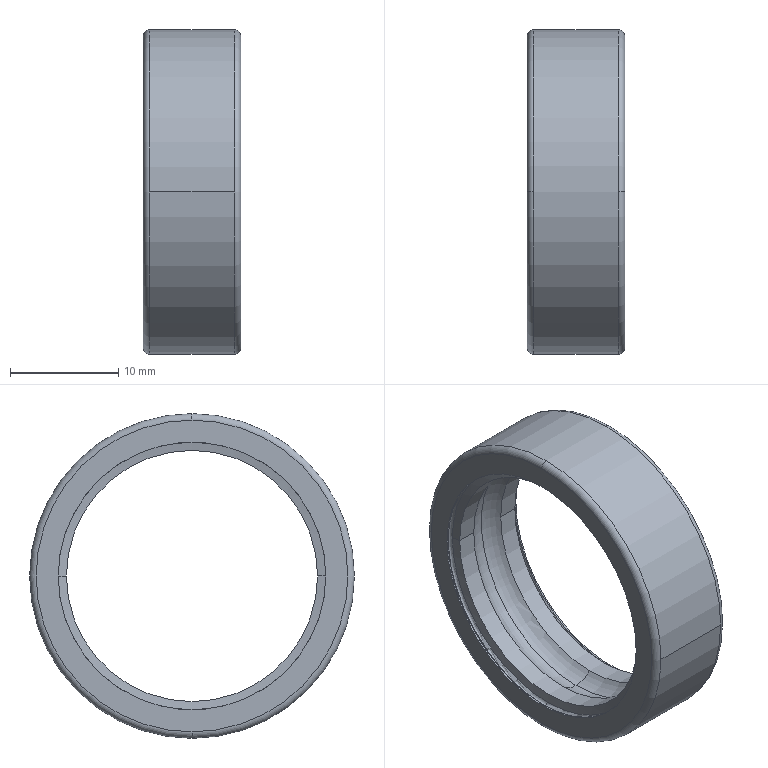Part | SolidWorks | features BaseBody 1 | 1 solid | 32 faces | box 9 x 30 x 30 mm | volume 2282 mm3 | torus 16 | cylinder 10 | cone 4 | plane 2 | commonest cylinder face diameters 23.2 x4 24.72 x4 30 x2
STEP:
#1=CARTESIAN_POINT('',(8.544,0.,-12.664));
#2=VERTEX_POINT('',#1);
#3=CARTESIAN_POINT('',(8.544,0.,12.664));
#4=VERTEX_POINT('',#3);
#5=CARTESIAN_POINT('',(8.544,0.,0.));
#6=DIRECTION('',(1.,0.,0.));
#7=DIRECTION('',(0.,0.,1.));
#8=AXIS2_PLACEMENT_3D('',#5,#6,#7);
#9=CIRCLE('',#8,12.664);
#10=EDGE_CURVE('',#2,#4,#9,.T.);
#11=ORIENTED_EDGE('',*,*,#10,.T.);
#12=CARTESIAN_POINT('',(8.245,0.,12.413));
#13=VERTEX_POINT('',#12);
#14=CARTESIAN_POINT('',(8.544,0.,12.36));
#15=DIRECTION('',(0.,-1.,0.));
#16=DIRECTION('',(0.,0.,1.));
#17=AXIS2_PLACEMENT_3D('',#14,#15,#16);
#18=CIRCLE('',#17,0.304);
#19=EDGE_CURVE('',#4,#13,#18,.T.);
#20=ORIENTED_EDGE('',*,*,#19,.T.);
#21=CARTESIAN_POINT('',(8.245,12.413,0.));
#22=VERTEX_POINT('',#21);
#23=CARTESIAN_POINT('',(8.245,0.,0.));
#24=DIRECTION('',(1.,0.,0.));
#25=DIRECTION('',(0.,1.,0.));
#26=AXIS2_PLACEMENT_3D('',#23,#24,#25);
#27=CIRCLE('',#26,12.413);
#28=EDGE_CURVE('',#22,#13,#27,.T.);
#29=ORIENTED_EDGE('',*,*,#28,.F.);
#30=CARTESIAN_POINT('',(8.245,0.,-12.413));
#31=VERTEX_POINT('',#30);
#32=CARTESIAN_POINT('',(8.245,0.,0.));
#33=DIRECTION('',(1.,0.,0.));
#34=DIRECTION('',(0.,1.,0.));
#35=AXIS2_PLACEMENT_3D('',#32,#33,#34);
#36=CIRCLE('',#35,12.413);
#37=EDGE_CURVE('',#31,#22,#36,.T.);
#38=ORIENTED_EDGE('',*,*,#37,.F.);
#39=CARTESIAN_POINT('',(8.544,0.,-12.36));
#40=DIRECTION('',(0.,-1.,0.));
#41=DIRECTION('',(0.,0.,-1.));
#42=AXIS2_PLACEMENT_3D('',#39,#40,#41);
#43=CIRCLE('',#42,0.304);
#44=EDGE_CURVE('',#31,#2,#43,.T.);
#45=ORIENTED_EDGE('',*,*,#44,.T.);
#46=EDGE_LOOP('',(#11,#20,#29,#38,#45));
#47=FACE_OUTER_BOUND('',#46,.T.);
#48=CARTESIAN_POINT('',(8.544,0.,0.));
#49=DIRECTION('',(1.,0.,0.));
#50=DIRECTION('',(0.,0.,-1.));
#51=AXIS2_PLACEMENT_3D('',#48,#49,#50);
#52=TOROIDAL_SURFACE('',#51,12.36,0.304);
#53=ADVANCED_FACE('',(#47),#52,.F.);
#54=CARTESIAN_POINT('',(8.848,12.36,0.));
#55=VERTEX_POINT('',#54);
#56=CARTESIAN_POINT('',(9.,12.36,0.));
#57=VERTEX_POINT('',#56);
#58=CARTESIAN_POINT('',(8.924,12.36,0.));
#59=DIRECTION('',(1.,0.,0.));
#60=VECTOR('',#59,1000.);
#61=LINE('',#58,#60);
#62=EDGE_CURVE('',#55,#57,#61,.T.);
#63=ORIENTED_EDGE('',*,*,#62,.T.);
#64=CARTESIAN_POINT('',(9.,-12.36,0.));
#65=VERTEX_POINT('',#64);
#66=CARTESIAN_POINT('',(9.,0.,0.));
#67=DIRECTION('',(1.,0.,0.));
#68=DIRECTION('',(0.,1.,0.));
#69=AXIS2_PLACEMENT_3D('',#66,#67,#68);
#70=CIRCLE('',#69,12.36);
#71=EDGE_CURVE('',#57,#65,#70,.T.);
#72=ORIENTED_EDGE('',*,*,#71,.T.);
#73=CARTESIAN_POINT('',(8.848,-12.36,0.));
#74=VERTEX_POINT('',#73);
#75=CARTESIAN_POINT('',(8.924,-12.36,0.));
#76=DIRECTION('',(-1.,0.,0.));
#77=VECTOR('',#76,1000.);
#78=LINE('',#75,#77);
#79=EDGE_CURVE('',#65,#74,#78,.T.);
#80=ORIENTED_EDGE('',*,*,#79,.T.);
#81=CARTESIAN_POINT('',(8.848,0.,12.36));
#82=VERTEX_POINT('',#81);
#83=CARTESIAN_POINT('',(8.848,0.,0.));
#84=DIRECTION('',(1.,0.,0.));
#85=DIRECTION('',(0.,1.,0.));
#86=AXIS2_PLACEMENT_3D('',#83,#84,#85);
#87=CIRCLE('',#86,12.36);
#88=EDGE_CURVE('',#82,#74,#87,.T.);
#89=ORIENTED_EDGE('',*,*,#88,.F.);
#90=CARTESIAN_POINT('',(8.848,0.,0.));
#91=DIRECTION('',(1.,0.,0.));
#92=DIRECTION('',(0.,1.,0.));
#93=AXIS2_PLACEMENT_3D('',#90,#91,#92);
#94=CIRCLE('',#93,12.36);
#95=EDGE_CURVE('',#55,#82,#94,.T.);
#96=ORIENTED_EDGE('',*,*,#95,.F.);
#97=EDGE_LOOP('',(#63,#72,#80,#89,#96));
#98=FACE_OUTER_BOUND('',#97,.T.);
#99=CARTESIAN_POINT('',(8.924,0.,0.));
#100=DIRECTION('',(1.,0.,0.));
#101=DIRECTION('',(0.,1.,0.));
#102=AXIS2_PLACEMENT_3D('',#99,#100,#101);
#103=CYLINDRICAL_SURFACE('',#102,12.36);
#104=ADVANCED_FACE('',(#98),#103,.F.);
#105=ORIENTED_EDGE('',*,*,#71,.F.);
#106=CARTESIAN_POINT('',(9.,0.,0.));
#107=DIRECTION('',(1.,0.,0.));
#108=DIRECTION('',(0.,1.,0.));
#109=AXIS2_PLACEMENT_3D('',#106,#107,#108);
#110=CIRCLE('',#109,12.36);
#111=EDGE_CURVE('',#65,#57,#110,.T.);
#112=ORIENTED_EDGE('',*,*,#111,.F.);
#113=EDGE_LOOP('',(#105,#112));
#114=FACE_BOUND('',#113,.T.);
#115=CARTESIAN_POINT('',(9.,0.,14.4));
#116=VERTEX_POINT('',#115);
#117=CARTESIAN_POINT('',(9.,0.,-14.4));
#118=VERTEX_POINT('',#117);
#119=CARTESIAN_POINT('',(9.,0.,0.));
#120=DIRECTION('',(1.,0.,0.));
#121=DIRECTION('',(0.,1.,0.));
#122=AXIS2_PLACEMENT_3D('',#119,#120,#121);
#123=CIRCLE('',#122,14.4);
#124=EDGE_CURVE('',#116,#118,#123,.T.);
#125=ORIENTED_EDGE('',*,*,#124,.T.);
#126=CARTESIAN_POINT('',(9.,0.,0.));
#127=DIRECTION('',(1.,0.,0.));
#128=DIRECTION('',(0.,1.,0.));
#129=AXIS2_PLACEMENT_3D('',#126,#127,#128);
#130=CIRCLE('',#129,14.4);
#131=EDGE_CURVE('',#118,#116,#130,.T.);
#132=ORIENTED_EDGE('',*,*,#131,.T.);
#133=EDGE_LOOP('',(#125,#132));
#134=FACE_OUTER_BOUND('',#133,.T.);
#135=CARTESIAN_POINT('',(9.,13.38,0.));
#136=DIRECTION('',(1.,0.,0.));
#137=DIRECTION('',(0.,1.,0.));
#138=AXIS2_PLACEMENT_3D('',#135,#136,#137);
#139=PLANE('',#138);
#140=ADVANCED_FACE('',(#114,#134),#139,.T.);
#141=CARTESIAN_POINT('',(8.4,0.,-15.));
#142=VERTEX_POINT('',#141);
#143=CARTESIAN_POINT('',(8.4,0.,-14.4));
#144=DIRECTION('',(0.,-1.,0.));
#145=DIRECTION('',(0.,0.,-1.));
#146=AXIS2_PLACEMENT_3D('',#143,#144,#145);
#147=CIRCLE('',#146,0.6);
#148=EDGE_CURVE('',#142,#118,#147,.T.);
#149=ORIENTED_EDGE('',*,*,#148,.T.);
#150=ORIENTED_EDGE('',*,*,#124,.F.);
#151=CARTESIAN_POINT('',(8.4,0.,15.));
#152=VERTEX_POINT('',#151);
#153=CARTESIAN_POINT('',(8.4,0.,14.4));
#154=DIRECTION('',(0.,-1.,0.));
#155=DIRECTION('',(0.,0.,1.));
#156=AXIS2_PLACEMENT_3D('',#153,#154,#155);
#157=CIRCLE('',#156,0.6);
#158=EDGE_CURVE('',#116,#152,#157,.T.);
#159=ORIENTED_EDGE('',*,*,#158,.T.);
#160=CARTESIAN_POINT('',(8.4,-15.,0.));
#161=VERTEX_POINT('',#160);
#162=CARTESIAN_POINT('',(8.4,0.,0.));
#163=DIRECTION('',(1.,0.,0.));
#164=DIRECTION('',(0.,1.,0.));
#165=AXIS2_PLACEMENT_3D('',#162,#163,#164);
#166=CIRCLE('',#165,15.);
#167=EDGE_CURVE('',#152,#161,#166,.T.);
#168=ORIENTED_EDGE('',*,*,#167,.T.);
#169=CARTESIAN_POINT('',(8.4,0.,0.));
#170=DIRECTION('',(1.,0.,0.));
#171=DIRECTION('',(0.,1.,0.));
#172=AXIS2_PLACEMENT_3D('',#169,#170,#171);
#173=CIRCLE('',#172,15.);
#174=EDGE_CURVE('',#161,#142,#173,.T.);
#175=ORIENTED_EDGE('',*,*,#174,.T.);
#176=EDGE_LOOP('',(#149,#150,#159,#168,#175));
#177=FACE_OUTER_BOUND('',#176,.T.);
#178=CARTESIAN_POINT('',(8.4,0.,0.));
#179=DIRECTION('',(1.,0.,0.));
#180=DIRECTION('',(0.,0.,-1.));
#181=AXIS2_PLACEMENT_3D('',#178,#179,#180);
#182=TOROIDAL_SURFACE('',#181,14.4,0.6);
#183=ADVANCED_FACE('',(#177),#182,.T.);
#184=CARTESIAN_POINT('',(0.6,15.,0.));
#185=VERTEX_POINT('',#184);
#186=CARTESIAN_POINT('',(8.4,15.,0.));
#187=VERTEX_POINT('',#186);
#188=CARTESIAN_POINT('',(4.5,15.,0.));
#189=DIRECTION('',(1.,0.,0.));
#190=VECTOR('',#189,1000.);
#191=LINE('',#188,#190);
#192=EDGE_CURVE('',#185,#187,#191,.T.);
#193=ORIENTED_EDGE('',*,*,#192,.T.);
#194=CARTESIAN_POINT('',(8.4,0.,0.));
#195=DIRECTION('',(1.,0.,0.));
#196=DIRECTION('',(0.,1.,0.));
#197=AXIS2_PLACEMENT_3D('',#194,#195,#196);
#198=CIRCLE('',#197,15.);
#199=EDGE_CURVE('',#142,#187,#198,.T.);
#200=ORIENTED_EDGE('',*,*,#199,.F.);
#201=ORIENTED_EDGE('',*,*,#174,.F.);
#202=CARTESIAN_POINT('',(0.6,-15.,0.));
#203=VERTEX_POINT('',#202);
#204=CARTESIAN_POINT('',(4.5,-15.,0.));
#205=DIRECTION('',(-1.,0.,0.));
#206=VECTOR('',#205,1000.);
#207=LINE('',#204,#206);
#208=EDGE_CURVE('',#161,#203,#207,.T.);
#209=ORIENTED_EDGE('',*,*,#208,.T.);
#210=CARTESIAN_POINT('',(0.6,0.,-15.));
#211=VERTEX_POINT('',#210);
#212=CARTESIAN_POINT('',(0.6,0.,0.));
#213=DIRECTION('',(1.,0.,0.));
#214=DIRECTION('',(0.,1.,0.));
#215=AXIS2_PLACEMENT_3D('',#212,#213,#214);
#216=CIRCLE('',#215,15.);
#217=EDGE_CURVE('',#203,#211,#216,.T.);
#218=ORIENTED_EDGE('',*,*,#217,.T.);
#219=CARTESIAN_POINT('',(0.6,0.,0.));
#220=DIRECTION('',(1.,0.,0.));
#221=DIRECTION('',(0.,1.,0.));
#222=AXIS2_PLACEMENT_3D('',#219,#220,#221);
#223=CIRCLE('',#222,15.);
#224=EDGE_CURVE('',#211,#185,#223,.T.);
#225=ORIENTED_EDGE('',*,*,#224,.T.);
#226=EDGE_LOOP('',(#193,#200,#201,#209,#218,#225));
#227=FACE_OUTER_BOUND('',#226,.T.);
#228=CARTESIAN_POINT('',(4.5,0.,0.));
#229=DIRECTION('',(1.,0.,0.));
#230=DIRECTION('',(0.,1.,0.));
#231=AXIS2_PLACEMENT_3D('',#228,#229,#230);
#232=CYLINDRICAL_SURFACE('',#231,15.);
#233=ADVANCED_FACE('',(#227),#232,.T.);
#234=CARTESIAN_POINT('',(0.,0.,-14.4));
#235=VERTEX_POINT('',#234);
#236=CARTESIAN_POINT('',(0.6,0.,-14.4));
#237=DIRECTION('',(0.,-1.,0.));
#238=DIRECTION('',(0.,0.,-1.));
#239=AXIS2_PLACEMENT_3D('',#236,#237,#238);
#240=CIRCLE('',#239,0.6);
#241=EDGE_CURVE('',#235,#211,#240,.T.);
#242=ORIENTED_EDGE('',*,*,#241,.T.);
#243=ORIENTED_EDGE('',*,*,#217,.F.);
#244=CARTESIAN_POINT('',(0.6,0.,15.));
#245=VERTEX_POINT('',#244);
#246=CARTESIAN_POINT('',(0.6,0.,0.));
#247=DIRECTION('',(1.,0.,0.));
#248=DIRECTION('',(0.,1.,0.));
#249=AXIS2_PLACEMENT_3D('',#246,#247,#248);
#250=CIRCLE('',#249,15.);
#251=EDGE_CURVE('',#245,#203,#250,.T.);
#252=ORIENTED_EDGE('',*,*,#251,.F.);
#253=CARTESIAN_POINT('',(0.,0.,14.4));
#254=VERTEX_POINT('',#253);
#255=CARTESIAN_POINT('',(0.6,0.,14.4));
#256=DIRECTION('',(0.,-1.,0.));
#257=DIRECTION('',(0.,0.,1.));
#258=AXIS2_PLACEMENT_3D('',#255,#256,#257);
#259=CIRCLE('',#258,0.6);
#260=EDGE_CURVE('',#245,#254,#259,.T.);
#261=ORIENTED_EDGE('',*,*,#260,.T.);
#262=CARTESIAN_POINT('',(0.,0.,0.));
#263=DIRECTION('',(1.,0.,0.));
#264=DIRECTION('',(0.,1.,0.));
#265=AXIS2_PLACEMENT_3D('',#262,#263,#264);
#266=CIRCLE('',#265,14.4);
#267=EDGE_CURVE('',#254,#235,#266,.T.);
#268=ORIENTED_EDGE('',*,*,#267,.T.);
#269=EDGE_LOOP('',(#242,#243,#252,#261,#268));
#270=FACE_OUTER_BOUND('',#269,.T.);
#271=CARTESIAN_POINT('',(0.6,0.,0.));
#272=DIRECTION('',(1.,0.,0.));
#273=DIRECTION('',(0.,0.,-1.));
#274=AXIS2_PLACEMENT_3D('',#271,#272,#273);
#275=TOROIDAL_SURFACE('',#274,14.4,0.6);
#276=ADVANCED_FACE('',(#270),#275,.T.);
#277=CARTESIAN_POINT('',(0.,12.36,0.));
#278=VERTEX_POINT('',#277);
#279=CARTESIAN_POINT('',(0.,-12.36,0.));
#280=VERTEX_POINT('',#279);
#281=CARTESIAN_POINT('',(0.,0.,0.));
#282=DIRECTION('',(1.,0.,0.));
#283=DIRECTION('',(0.,1.,0.));
#284=AXIS2_PLACEMENT_3D('',#281,#282,#283);
#285=CIRCLE('',#284,12.36);
#286=EDGE_CURVE('',#278,#280,#285,.T.);
#287=ORIENTED_EDGE('',*,*,#286,.T.);
#288=CARTESIAN_POINT('',(0.,0.,0.));
#289=DIRECTION('',(1.,0.,0.));
#290=DIRECTION('',(0.,1.,0.));
#291=AXIS2_PLACEMENT_3D('',#288,#289,#290);
#292=CIRCLE('',#291,12.36);
#293=EDGE_CURVE('',#280,#278,#292,.T.);
#294=ORIENTED_EDGE('',*,*,#293,.T.);
#295=EDGE_LOOP('',(#287,#294));
#296=FACE_BOUND('',#295,.T.);
#297=CARTESIAN_POINT('',(0.,0.,0.));
#298=DIRECTION('',(1.,0.,0.));
#299=DIRECTION('',(0.,1.,0.));
#300=AXIS2_PLACEMENT_3D('',#297,#298,#299);
#301=CIRCLE('',#300,14.4);
#302=EDGE_CURVE('',#235,#254,#301,.T.);
#303=ORIENTED_EDGE('',*,*,#302,.F.);
#304=ORIENTED_EDGE('',*,*,#267,.F.);
#305=EDGE_LOOP('',(#303,#304));
#306=FACE_OUTER_BOUND('',#305,.T.);
#307=CARTESIAN_POINT('',(0.,13.38,0.));
#308=DIRECTION('',(-1.,0.,0.));
#309=DIRECTION('',(0.,0.,1.));
#310=AXIS2_PLACEMENT_3D('',#307,#308,#309);
#311=PLANE('',#310);
#312=ADVANCED_FACE('',(#296,#306),#311,.T.);
#313=CARTESIAN_POINT('',(0.152,12.36,0.));
#314=VERTEX_POINT('',#313);
#315=CARTESIAN_POINT('',(0.076,12.36,0.));
#316=DIRECTION('',(1.,0.,0.));
#317=VECTOR('',#316,1000.);
#318=LINE('',#315,#317);
#319=EDGE_CURVE('',#278,#314,#318,.T.);
#320=ORIENTED_EDGE('',*,*,#319,.T.);
#321=CARTESIAN_POINT('',(0.152,0.,12.36));
#322=VERTEX_POINT('',#321);
#323=CARTESIAN_POINT('',(0.152,0.,0.));
#324=DIRECTION('',(1.,0.,0.));
#325=DIRECTION('',(0.,1.,0.));
#326=AXIS2_PLACEMENT_3D('',#323,#324,#325);
#327=CIRCLE('',#326,12.36);
#328=EDGE_CURVE('',#314,#322,#327,.T.);
#329=ORIENTED_EDGE('',*,*,#328,.T.);
#330=CARTESIAN_POINT('',(0.152,-12.36,0.));
#331=VERTEX_POINT('',#330);
#332=CARTESIAN_POINT('',(0.152,0.,0.));
#333=DIRECTION('',(1.,0.,0.));
#334=DIRECTION('',(0.,1.,0.));
#335=AXIS2_PLACEMENT_3D('',#332,#333,#334);
#336=CIRCLE('',#335,12.36);
#337=EDGE_CURVE('',#322,#331,#336,.T.);
#338=ORIENTED_EDGE('',*,*,#337,.T.);
#339=CARTESIAN_POINT('',(0.076,-12.36,0.));
#340=DIRECTION('',(-1.,0.,0.));
#341=VECTOR('',#340,1000.);
#342=LINE('',#339,#341);
#343=EDGE_CURVE('',#331,#280,#342,.T.);
#344=ORIENTED_EDGE('',*,*,#343,.T.);
#345=ORIENTED_EDGE('',*,*,#286,.F.);
#346=EDGE_LOOP('',(#320,#329,#338,#344,#345));
#347=FACE_OUTER_BOUND('',#346,.T.);
#348=CARTESIAN_POINT('',(0.076,0.,0.));
#349=DIRECTION('',(1.,0.,0.));
#350=DIRECTION('',(0.,1.,0.));
#351=AXIS2_PLACEMENT_3D('',#348,#349,#350);
#352=CYLINDRICAL_SURFACE('',#351,12.36);
#353=ADVANCED_FACE('',(#347),#352,.F.);
#354=CARTESIAN_POINT('',(0.456,0.,-12.664));
#355=VERTEX_POINT('',#354);
#356=CARTESIAN_POINT('',(0.456,0.,12.664));
#357=VERTEX_POINT('',#356);
#358=CARTESIAN_POINT('',(0.456,0.,0.));
#359=DIRECTION('',(1.,0.,0.));
#360=DIRECTION('',(0.,0.,1.));
#361=AXIS2_PLACEMENT_3D('',#358,#359,#360);
#362=CIRCLE('',#361,12.664);
#363=EDGE_CURVE('',#355,#357,#362,.T.);
#364=ORIENTED_EDGE('',*,*,#363,.T.);
#365=CARTESIAN_POINT('',(0.456,0.,12.36));
#366=DIRECTION('',(0.,-1.,0.));
#367=DIRECTION('',(0.,0.,1.));
#368=AXIS2_PLACEMENT_3D('',#365,#366,#367);
#369=CIRCLE('',#368,0.304);
#370=EDGE_CURVE('',#357,#322,#369,.T.);
#371=ORIENTED_EDGE('',*,*,#370,.T.);
#372=ORIENTED_EDGE('',*,*,#328,.F.);
#373=CARTESIAN_POINT('',(0.152,0.,-12.36));
#374=VERTEX_POINT('',#373);
#375=CARTESIAN_POINT('',(0.152,0.,0.));
#376=DIRECTION('',(1.,0.,0.));
#377=DIRECTION('',(0.,1.,0.));
#378=AXIS2_PLACEMENT_3D('',#375,#376,#377);
#379=CIRCLE('',#378,12.36);
#380=EDGE_CURVE('',#374,#314,#379,.T.);
#381=ORIENTED_EDGE('',*,*,#380,.F.);
#382=CARTESIAN_POINT('',(0.456,0.,-12.36));
#383=DIRECTION('',(0.,-1.,0.));
#384=DIRECTION('',(0.,0.,-1.));
#385=AXIS2_PLACEMENT_3D('',#382,#383,#384);
#386=CIRCLE('',#385,0.304);
#387=EDGE_CURVE('',#374,#355,#386,.T.);
#388=ORIENTED_EDGE('',*,*,#387,.T.);
#389=EDGE_LOOP('',(#364,#371,#372,#381,#388));
#390=FACE_OUTER_BOUND('',#389,.T.);
#391=CARTESIAN_POINT('',(0.456,0.,0.));
#392=DIRECTION('',(1.,0.,0.));
#393=DIRECTION('',(0.,0.,-1.));
#394=AXIS2_PLACEMENT_3D('',#391,#392,#393);
#395=TOROIDAL_SURFACE('',#394,12.36,0.304);
#396=ADVANCED_FACE('',(#390),#395,.F.);
#397=CARTESIAN_POINT('',(0.7554,12.413,0.));
#398=VERTEX_POINT('',#397);
#399=CARTESIAN_POINT('',(0.8987,11.6,0.));
#400=VERTEX_POINT('',#399);
#401=CARTESIAN_POINT('',(0.827,12.006,0.));
#402=DIRECTION('',(0.1736,-0.9848,0.));
#403=VECTOR('',#402,1000.);
#404=LINE('',#401,#403);
#405=EDGE_CURVE('',#398,#400,#404,.T.);
#406=ORIENTED_EDGE('',*,*,#405,.T.);
#407=CARTESIAN_POINT('',(0.8987,-11.6,0.));
#408=VERTEX_POINT('',#407);
#409=CARTESIAN_POINT('',(0.8987,0.,0.));
#410=DIRECTION('',(1.,0.,0.));
#411=DIRECTION('',(0.,1.,0.));
#412=AXIS2_PLACEMENT_3D('',#409,#410,#411);
#413=CIRCLE('',#412,11.6);
#414=EDGE_CURVE('',#400,#408,#413,.T.);
#415=ORIENTED_EDGE('',*,*,#414,.T.);
#416=CARTESIAN_POINT('',(0.7554,-12.413,0.));
#417=VERTEX_POINT('',#416);
#418=CARTESIAN_POINT('',(0.827,-12.006,0.));
#419=DIRECTION('',(-0.1736,-0.9848,0.));
#420=VECTOR('',#419,1000.);
#421=LINE('',#418,#420);
#422=EDGE_CURVE('',#408,#417,#421,.T.);
#423=ORIENTED_EDGE('',*,*,#422,.T.);
#424=CARTESIAN_POINT('',(0.7554,0.,12.413));
#425=VERTEX_POINT('',#424);
#426=CARTESIAN_POINT('',(0.7554,0.,0.));
#427=DIRECTION('',(1.,0.,0.));
#428=DIRECTION('',(0.,1.,0.));
#429=AXIS2_PLACEMENT_3D('',#426,#427,#428);
#430=CIRCLE('',#429,12.413);
#431=EDGE_CURVE('',#425,#417,#430,.T.);
#432=ORIENTED_EDGE('',*,*,#431,.F.);
#433=CARTESIAN_POINT('',(0.7554,0.,0.));
#434=DIRECTION('',(1.,0.,0.));
#435=DIRECTION('',(0.,1.,0.));
#436=AXIS2_PLACEMENT_3D('',#433,#434,#435);
#437=CIRCLE('',#436,12.413);
#438=EDGE_CURVE('',#398,#425,#437,.T.);
#439=ORIENTED_EDGE('',*,*,#438,.F.);
#440=EDGE_LOOP('',(#406,#415,#423,#432,#439));
#441=FACE_OUTER_BOUND('',#440,.T.);
#442=CARTESIAN_POINT('',(0.827,0.,0.));
#443=DIRECTION('',(-1.,0.,0.));
#444=DIRECTION('',(0.,1.,0.));
#445=AXIS2_PLACEMENT_3D('',#442,#443,#444);
#446=CONICAL_SURFACE('',#445,12.006,1.396);
#447=ADVANCED_FACE('',(#441),#446,.F.);
#448=CARTESIAN_POINT('',(2.737,11.6,0.));
#449=VERTEX_POINT('',#448);
#450=CARTESIAN_POINT('',(1.818,11.6,0.));
#451=DIRECTION('',(1.,0.,0.));
#452=VECTOR('',#451,1000.);
#453=LINE('',#450,#452);
#454=EDGE_CURVE('',#400,#449,#453,.T.);
#455=ORIENTED_EDGE('',*,*,#454,.T.);
#456=CARTESIAN_POINT('',(2.737,0.,11.6));
#457=VERTEX_POINT('',#456);
#458=CARTESIAN_POINT('',(2.737,0.,0.));
#459=DIRECTION('',(1.,0.,0.));
#460=DIRECTION('',(0.,1.,0.));
#461=AXIS2_PLACEMENT_3D('',#458,#459,#460);
#462=CIRCLE('',#461,11.6);
#463=EDGE_CURVE('',#449,#457,#462,.T.);
#464=ORIENTED_EDGE('',*,*,#463,.T.);
#465=CARTESIAN_POINT('',(2.737,-11.6,0.));
#466=VERTEX_POINT('',#465);
#467=CARTESIAN_POINT('',(2.737,0.,0.));
#468=DIRECTION('',(1.,0.,0.));
#469=DIRECTION('',(0.,1.,0.));
#470=AXIS2_PLACEMENT_3D('',#467,#468,#469);
#471=CIRCLE('',#470,11.6);
#472=EDGE_CURVE('',#457,#466,#471,.T.);
#473=ORIENTED_EDGE('',*,*,#472,.T.);
#474=CARTESIAN_POINT('',(1.818,-11.6,0.));
#475=DIRECTION('',(-1.,0.,0.));
#476=VECTOR('',#475,1000.);
#477=LINE('',#474,#476);
#478=EDGE_CURVE('',#466,#408,#477,.T.);
#479=ORIENTED_EDGE('',*,*,#478,.T.);
#480=ORIENTED_EDGE('',*,*,#414,.F.);
#481=EDGE_LOOP('',(#455,#464,#473,#479,#480));
#482=FACE_OUTER_BOUND('',#481,.T.);
#483=CARTESIAN_POINT('',(1.818,0.,0.));
#484=DIRECTION('',(1.,0.,0.));
#485=DIRECTION('',(0.,1.,0.));
#486=AXIS2_PLACEMENT_3D('',#483,#484,#485);
#487=CYLINDRICAL_SURFACE('',#486,11.6);
#488=ADVANCED_FACE('',(#482),#487,.F.);
#489=CARTESIAN_POINT('',(4.5,0.,-12.381));
#490=VERTEX_POINT('',#489);
#491=CARTESIAN_POINT('',(4.5,0.,12.381));
#492=VERTEX_POINT('',#491);
#493=CARTESIAN_POINT('',(4.5,0.,0.));
#494=DIRECTION('',(1.,0.,0.));
#495=DIRECTION('',(0.,0.,1.));
#496=AXIS2_PLACEMENT_3D('',#493,#494,#495);
#497=CIRCLE('',#496,12.381);
#498=EDGE_CURVE('',#490,#492,#497,.T.);
#499=ORIENTED_EDGE('',*,*,#498,.T.);
#500=CARTESIAN_POINT('',(4.5,0.,10.));
#501=DIRECTION('',(0.,-1.,0.));
#502=DIRECTION('',(0.,0.,1.));
#503=AXIS2_PLACEMENT_3D('',#500,#501,#502);
#504=CIRCLE('',#503,2.381);
#505=EDGE_CURVE('',#492,#457,#504,.T.);
#506=ORIENTED_EDGE('',*,*,#505,.T.);
#507=ORIENTED_EDGE('',*,*,#463,.F.);
#508=CARTESIAN_POINT('',(2.737,0.,-11.6));
#509=VERTEX_POINT('',#508);
#510=CARTESIAN_POINT('',(2.737,0.,0.));
#511=DIRECTION('',(1.,0.,0.));
#512=DIRECTION('',(0.,1.,0.));
#513=AXIS2_PLACEMENT_3D('',#510,#511,#512);
#514=CIRCLE('',#513,11.6);
#515=EDGE_CURVE('',#509,#449,#514,.T.);
#516=ORIENTED_EDGE('',*,*,#515,.F.);
#517=CARTESIAN_POINT('',(4.5,0.,-10.));
#518=DIRECTION('',(0.,-1.,0.));
#519=DIRECTION('',(0.,0.,-1.));
#520=AXIS2_PLACEMENT_3D('',#517,#518,#519);
#521=CIRCLE('',#520,2.381);
#522=EDGE_CURVE('',#509,#490,#521,.T.);
#523=ORIENTED_EDGE('',*,*,#522,.T.);
#524=EDGE_LOOP('',(#499,#506,#507,#516,#523));
#525=FACE_OUTER_BOUND('',#524,.T.);
#526=CARTESIAN_POINT('',(4.5,0.,0.));
#527=DIRECTION('',(1.,0.,0.));
#528=DIRECTION('',(0.,0.,-1.));
#529=AXIS2_PLACEMENT_3D('',#526,#527,#528);
#530=TOROIDAL_SURFACE('',#529,10.,2.381);
#531=ADVANCED_FACE('',(#525),#530,.F.);
#532=CARTESIAN_POINT('',(6.263,11.6,0.));
#533=VERTEX_POINT('',#532);
#534=CARTESIAN_POINT('',(8.101,11.6,0.));
#535=VERTEX_POINT('',#534);
#536=CARTESIAN_POINT('',(7.182,11.6,0.));
#537=DIRECTION('',(1.,0.,0.));
#538=VECTOR('',#537,1000.);
#539=LINE('',#536,#538);
#540=EDGE_CURVE('',#533,#535,#539,.T.);
#541=ORIENTED_EDGE('',*,*,#540,.T.);
#542=CARTESIAN_POINT('',(8.101,-11.6,0.));
#543=VERTEX_POINT('',#542);
#544=CARTESIAN_POINT('',(8.101,0.,0.));
#545=DIRECTION('',(1.,0.,0.));
#546=DIRECTION('',(0.,1.,0.));
#547=AXIS2_PLACEMENT_3D('',#544,#545,#546);
#548=CIRCLE('',#547,11.6);
#549=EDGE_CURVE('',#535,#543,#548,.T.);
#550=ORIENTED_EDGE('',*,*,#549,.T.);
#551=CARTESIAN_POINT('',(6.263,-11.6,0.));
#552=VERTEX_POINT('',#551);
#553=CARTESIAN_POINT('',(7.182,-11.6,0.));
#554=DIRECTION('',(-1.,0.,0.));
#555=VECTOR('',#554,1000.);
#556=LINE('',#553,#555);
#557=EDGE_CURVE('',#543,#552,#556,.T.);
#558=ORIENTED_EDGE('',*,*,#557,.T.);
#559=CARTESIAN_POINT('',(6.263,0.,11.6));
#560=VERTEX_POINT('',#559);
#561=CARTESIAN_POINT('',(6.263,0.,0.));
#562=DIRECTION('',(1.,0.,0.));
#563=DIRECTION('',(0.,1.,0.));
#564=AXIS2_PLACEMENT_3D('',#561,#562,#563);
#565=CIRCLE('',#564,11.6);
#566=EDGE_CURVE('',#560,#552,#565,.T.);
#567=ORIENTED_EDGE('',*,*,#566,.F.);
#568=CARTESIAN_POINT('',(6.263,0.,0.));
#569=DIRECTION('',(1.,0.,0.));
#570=DIRECTION('',(0.,1.,0.));
#571=AXIS2_PLACEMENT_3D('',#568,#569,#570);
#572=CIRCLE('',#571,11.6);
#573=EDGE_CURVE('',#533,#560,#572,.T.);
#574=ORIENTED_EDGE('',*,*,#573,.F.);
#575=EDGE_LOOP('',(#541,#550,#558,#567,#574));
#576=FACE_OUTER_BOUND('',#575,.T.);
#577=CARTESIAN_POINT('',(7.182,0.,0.));
#578=DIRECTION('',(1.,0.,0.));
#579=DIRECTION('',(0.,1.,0.));
#580=AXIS2_PLACEMENT_3D('',#577,#578,#579);
#581=CYLINDRICAL_SURFACE('',#580,11.6);
#582=ADVANCED_FACE('',(#576),#581,.F.);
#583=CARTESIAN_POINT('',(8.173,12.006,0.));
#584=DIRECTION('',(0.1736,0.9848,0.));
#585=VECTOR('',#584,1000.);
#586=LINE('',#583,#585);
#587=EDGE_CURVE('',#535,#22,#586,.T.);
#588=ORIENTED_EDGE('',*,*,#587,.T.);
#589=ORIENTED_EDGE('',*,*,#28,.T.);
#590=CARTESIAN_POINT('',(8.245,-12.413,0.));
#591=VERTEX_POINT('',#590);
#592=CARTESIAN_POINT('',(8.245,0.,0.));
#593=DIRECTION('',(1.,0.,0.));
#594=DIRECTION('',(0.,1.,0.));
#595=AXIS2_PLACEMENT_3D('',#592,#593,#594);
#596=CIRCLE('',#595,12.413);
#597=EDGE_CURVE('',#13,#591,#596,.T.);
#598=ORIENTED_EDGE('',*,*,#597,.T.);
#599=CARTESIAN_POINT('',(8.173,-12.006,0.));
#600=DIRECTION('',(-0.1736,0.9848,0.));
#601=VECTOR('',#600,1000.);
#602=LINE('',#599,#601);
#603=EDGE_CURVE('',#591,#543,#602,.T.);
#604=ORIENTED_EDGE('',*,*,#603,.T.);
#605=ORIENTED_EDGE('',*,*,#549,.F.);
#606=EDGE_LOOP('',(#588,#589,#598,#604,#605));
#607=FACE_OUTER_BOUND('',#606,.T.);
#608=CARTESIAN_POINT('',(8.173,0.,0.));
#609=DIRECTION('',(1.,0.,0.));
#610=DIRECTION('',(0.,1.,0.));
#611=AXIS2_PLACEMENT_3D('',#608,#609,#610);
#612=CONICAL_SURFACE('',#611,12.006,1.396);
#613=ADVANCED_FACE('',(#607),#612,.F.);
#614=ORIENTED_EDGE('',*,*,#587,.F.);
#615=CARTESIAN_POINT('',(8.101,0.,0.));
#616=DIRECTION('',(1.,0.,0.));
#617=DIRECTION('',(0.,1.,0.));
#618=AXIS2_PLACEMENT_3D('',#615,#616,#617);
#619=CIRCLE('',#618,11.6);
#620=EDGE_CURVE('',#543,#535,#619,.T.);
#621=ORIENTED_EDGE('',*,*,#620,.F.);
#622=ORIENTED_EDGE('',*,*,#603,.F.);
#623=CARTESIAN_POINT('',(8.245,0.,0.));
#624=DIRECTION('',(1.,0.,0.));
#625=DIRECTION('',(0.,1.,0.));
#626=AXIS2_PLACEMENT_3D('',#623,#624,#625);
#627=CIRCLE('',#626,12.413);
#628=EDGE_CURVE('',#591,#31,#627,.T.);
#629=ORIENTED_EDGE('',*,*,#628,.T.);
#630=ORIENTED_EDGE('',*,*,#37,.T.);
#631=EDGE_LOOP('',(#614,#621,#622,#629,#630));
#632=FACE_OUTER_BOUND('',#631,.T.);
#633=CARTESIAN_POINT('',(8.173,0.,0.));
#634=DIRECTION('',(1.,0.,0.));
#635=DIRECTION('',(0.,1.,0.));
#636=AXIS2_PLACEMENT_3D('',#633,#634,#635);
#637=CONICAL_SURFACE('',#636,12.006,1.396);
#638=ADVANCED_FACE('',(#632),#637,.F.);
#639=ORIENTED_EDGE('',*,*,#540,.F.);
#640=CARTESIAN_POINT('',(6.263,0.,-11.6));
#641=VERTEX_POINT('',#640);
#642=CARTESIAN_POINT('',(6.263,0.,0.));
#643=DIRECTION('',(1.,0.,0.));
#644=DIRECTION('',(0.,1.,0.));
#645=AXIS2_PLACEMENT_3D('',#642,#643,#644);
#646=CIRCLE('',#645,11.6);
#647=EDGE_CURVE('',#641,#533,#646,.T.);
#648=ORIENTED_EDGE('',*,*,#647,.F.);
#649=CARTESIAN_POINT('',(6.263,0.,0.));
#650=DIRECTION('',(1.,0.,0.));
#651=DIRECTION('',(0.,1.,0.));
#652=AXIS2_PLACEMENT_3D('',#649,#650,#651);
#653=CIRCLE('',#652,11.6);
#654=EDGE_CURVE('',#552,#641,#653,.T.);
#655=ORIENTED_EDGE('',*,*,#654,.F.);
#656=ORIENTED_EDGE('',*,*,#557,.F.);
#657=ORIENTED_EDGE('',*,*,#620,.T.);
#658=EDGE_LOOP('',(#639,#648,#655,#656,#657));
#659=FACE_OUTER_BOUND('',#658,.T.);
#660=CARTESIAN_POINT('',(7.182,0.,0.));
#661=DIRECTION('',(1.,0.,0.));
#662=DIRECTION('',(0.,1.,0.));
#663=AXIS2_PLACEMENT_3D('',#660,#661,#662);
#664=CYLINDRICAL_SURFACE('',#663,11.6);
#665=ADVANCED_FACE('',(#659),#664,.F.);
#666=CARTESIAN_POINT('',(4.5,0.,0.));
#667=DIRECTION('',(1.,0.,0.));
#668=DIRECTION('',(0.,0.,1.));
#669=AXIS2_PLACEMENT_3D('',#666,#667,#668);
#670=CIRCLE('',#669,12.381);
#671=EDGE_CURVE('',#492,#490,#670,.T.);
#672=ORIENTED_EDGE('',*,*,#671,.T.);
#673=ORIENTED_EDGE('',*,*,#522,.F.);
#674=CARTESIAN_POINT('',(2.737,0.,0.));
#675=DIRECTION('',(1.,0.,0.));
#676=DIRECTION('',(0.,1.,0.));
#677=AXIS2_PLACEMENT_3D('',#674,#675,#676);
#678=CIRCLE('',#677,11.6);
#679=EDGE_CURVE('',#466,#509,#678,.T.);
#680=ORIENTED_EDGE('',*,*,#679,.F.);
#681=ORIENTED_EDGE('',*,*,#472,.F.);
#682=ORIENTED_EDGE('',*,*,#505,.F.);
#683=EDGE_LOOP('',(#672,#673,#680,#681,#682));
#684=FACE_OUTER_BOUND('',#683,.T.);
#685=CARTESIAN_POINT('',(4.5,0.,0.));
#686=DIRECTION('',(1.,0.,0.));
#687=DIRECTION('',(0.,0.,-1.));
#688=AXIS2_PLACEMENT_3D('',#685,#686,#687);
#689=TOROIDAL_SURFACE('',#688,10.,2.381);
#690=ADVANCED_FACE('',(#684),#689,.F.);
#691=ORIENTED_EDGE('',*,*,#454,.F.);
#692=CARTESIAN_POINT('',(0.8987,0.,0.));
#693=DIRECTION('',(1.,0.,0.));
#694=DIRECTION('',(0.,1.,0.));
#695=AXIS2_PLACEMENT_3D('',#692,#693,#694);
#696=CIRCLE('',#695,11.6);
#697=EDGE_CURVE('',#408,#400,#696,.T.);
#698=ORIENTED_EDGE('',*,*,#697,.F.);
#699=ORIENTED_EDGE('',*,*,#478,.F.);
#700=ORIENTED_EDGE('',*,*,#679,.T.);
#701=ORIENTED_EDGE('',*,*,#515,.T.);
#702=EDGE_LOOP('',(#691,#698,#699,#700,#701));
#703=FACE_OUTER_BOUND('',#702,.T.);
#704=CARTESIAN_POINT('',(1.818,0.,0.));
#705=DIRECTION('',(1.,0.,0.));
#706=DIRECTION('',(0.,1.,0.));
#707=AXIS2_PLACEMENT_3D('',#704,#705,#706);
#708=CYLINDRICAL_SURFACE('',#707,11.6);
#709=ADVANCED_FACE('',(#703),#708,.F.);
#710=ORIENTED_EDGE('',*,*,#405,.F.);
#711=CARTESIAN_POINT('',(0.7554,0.,-12.413));
#712=VERTEX_POINT('',#711);
#713=CARTESIAN_POINT('',(0.7554,0.,0.));
#714=DIRECTION('',(1.,0.,0.));
#715=DIRECTION('',(0.,1.,0.));
#716=AXIS2_PLACEMENT_3D('',#713,#714,#715);
#717=CIRCLE('',#716,12.413);
#718=EDGE_CURVE('',#712,#398,#717,.T.);
#719=ORIENTED_EDGE('',*,*,#718,.F.);
#720=CARTESIAN_POINT('',(0.7554,0.,0.));
#721=DIRECTION('',(1.,0.,0.));
#722=DIRECTION('',(0.,1.,0.));
#723=AXIS2_PLACEMENT_3D('',#720,#721,#722);
#724=CIRCLE('',#723,12.413);
#725=EDGE_CURVE('',#417,#712,#724,.T.);
#726=ORIENTED_EDGE('',*,*,#725,.F.);
#727=ORIENTED_EDGE('',*,*,#422,.F.);
#728=ORIENTED_EDGE('',*,*,#697,.T.);
#729=EDGE_LOOP('',(#710,#719,#726,#727,#728));
#730=FACE_OUTER_BOUND('',#729,.T.);
#731=CARTESIAN_POINT('',(0.827,0.,0.));
#732=DIRECTION('',(-1.,0.,0.));
#733=DIRECTION('',(0.,1.,0.));
#734=AXIS2_PLACEMENT_3D('',#731,#732,#733);
#735=CONICAL_SURFACE('',#734,12.006,1.396);
#736=ADVANCED_FACE('',(#730),#735,.F.);
#737=CARTESIAN_POINT('',(0.456,0.,0.));
#738=DIRECTION('',(1.,0.,0.));
#739=DIRECTION('',(0.,0.,1.));
#740=AXIS2_PLACEMENT_3D('',#737,#738,#739);
#741=CIRCLE('',#740,12.664);
#742=EDGE_CURVE('',#357,#355,#741,.T.);
#743=ORIENTED_EDGE('',*,*,#742,.T.);
#744=ORIENTED_EDGE('',*,*,#387,.F.);
#745=CARTESIAN_POINT('',(0.152,0.,0.));
#746=DIRECTION('',(1.,0.,0.));
#747=DIRECTION('',(0.,1.,0.));
#748=AXIS2_PLACEMENT_3D('',#745,#746,#747);
#749=CIRCLE('',#748,12.36);
#750=EDGE_CURVE('',#331,#374,#749,.T.);
#751=ORIENTED_EDGE('',*,*,#750,.F.);
#752=ORIENTED_EDGE('',*,*,#337,.F.);
#753=ORIENTED_EDGE('',*,*,#370,.F.);
#754=EDGE_LOOP('',(#743,#744,#751,#752,#753));
#755=FACE_OUTER_BOUND('',#754,.T.);
#756=CARTESIAN_POINT('',(0.456,0.,0.));
#757=DIRECTION('',(1.,0.,0.));
#758=DIRECTION('',(0.,0.,-1.));
#759=AXIS2_PLACEMENT_3D('',#756,#757,#758);
#760=TOROIDAL_SURFACE('',#759,12.36,0.304);
#761=ADVANCED_FACE('',(#755),#760,.F.);
#762=ORIENTED_EDGE('',*,*,#319,.F.);
#763=ORIENTED_EDGE('',*,*,#293,.F.);
#764=ORIENTED_EDGE('',*,*,#343,.F.);
#765=ORIENTED_EDGE('',*,*,#750,.T.);
#766=ORIENTED_EDGE('',*,*,#380,.T.);
#767=EDGE_LOOP('',(#762,#763,#764,#765,#766));
#768=FACE_OUTER_BOUND('',#767,.T.);
#769=CARTESIAN_POINT('',(0.076,0.,0.));
#770=DIRECTION('',(1.,0.,0.));
#771=DIRECTION('',(0.,1.,0.));
#772=AXIS2_PLACEMENT_3D('',#769,#770,#771);
#773=CYLINDRICAL_SURFACE('',#772,12.36);
#774=ADVANCED_FACE('',(#768),#773,.F.);
#775=ORIENTED_EDGE('',*,*,#241,.F.);
#776=ORIENTED_EDGE('',*,*,#302,.T.);
#777=ORIENTED_EDGE('',*,*,#260,.F.);
#778=CARTESIAN_POINT('',(0.6,0.,0.));
#779=DIRECTION('',(1.,0.,0.));
#780=DIRECTION('',(0.,1.,0.));
#781=AXIS2_PLACEMENT_3D('',#778,#779,#780);
#782=CIRCLE('',#781,15.);
#783=EDGE_CURVE('',#185,#245,#782,.T.);
#784=ORIENTED_EDGE('',*,*,#783,.F.);
#785=ORIENTED_EDGE('',*,*,#224,.F.);
#786=EDGE_LOOP('',(#775,#776,#777,#784,#785));
#787=FACE_OUTER_BOUND('',#786,.T.);
#788=CARTESIAN_POINT('',(0.6,0.,0.));
#789=DIRECTION('',(1.,0.,0.));
#790=DIRECTION('',(0.,0.,-1.));
#791=AXIS2_PLACEMENT_3D('',#788,#789,#790);
#792=TOROIDAL_SURFACE('',#791,14.4,0.6);
#793=ADVANCED_FACE('',(#787),#792,.T.);
#794=ORIENTED_EDGE('',*,*,#192,.F.);
#795=ORIENTED_EDGE('',*,*,#783,.T.);
#796=ORIENTED_EDGE('',*,*,#251,.T.);
#797=ORIENTED_EDGE('',*,*,#208,.F.);
#798=ORIENTED_EDGE('',*,*,#167,.F.);
#799=CARTESIAN_POINT('',(8.4,0.,0.));
#800=DIRECTION('',(1.,0.,0.));
#801=DIRECTION('',(0.,1.,0.));
#802=AXIS2_PLACEMENT_3D('',#799,#800,#801);
#803=CIRCLE('',#802,15.);
#804=EDGE_CURVE('',#187,#152,#803,.T.);
#805=ORIENTED_EDGE('',*,*,#804,.F.);
#806=EDGE_LOOP('',(#794,#795,#796,#797,#798,#805));
#807=FACE_OUTER_BOUND('',#806,.T.);
#808=CARTESIAN_POINT('',(4.5,0.,0.));
#809=DIRECTION('',(1.,0.,0.));
#810=DIRECTION('',(0.,1.,0.));
#811=AXIS2_PLACEMENT_3D('',#808,#809,#810);
#812=CYLINDRICAL_SURFACE('',#811,15.);
#813=ADVANCED_FACE('',(#807),#812,.T.);
#814=ORIENTED_EDGE('',*,*,#148,.F.);
#815=ORIENTED_EDGE('',*,*,#199,.T.);
#816=ORIENTED_EDGE('',*,*,#804,.T.);
#817=ORIENTED_EDGE('',*,*,#158,.F.);
#818=ORIENTED_EDGE('',*,*,#131,.F.);
#819=EDGE_LOOP('',(#814,#815,#816,#817,#818));
#820=FACE_OUTER_BOUND('',#819,.T.);
#821=CARTESIAN_POINT('',(8.4,0.,0.));
#822=DIRECTION('',(1.,0.,0.));
#823=DIRECTION('',(0.,0.,-1.));
#824=AXIS2_PLACEMENT_3D('',#821,#822,#823);
#825=TOROIDAL_SURFACE('',#824,14.4,0.6);
#826=ADVANCED_FACE('',(#820),#825,.T.);
#827=ORIENTED_EDGE('',*,*,#62,.F.);
#828=CARTESIAN_POINT('',(8.848,0.,-12.36));
#829=VERTEX_POINT('',#828);
#830=CARTESIAN_POINT('',(8.848,0.,0.));
#831=DIRECTION('',(1.,0.,0.));
#832=DIRECTION('',(0.,1.,0.));
#833=AXIS2_PLACEMENT_3D('',#830,#831,#832);
#834=CIRCLE('',#833,12.36);
#835=EDGE_CURVE('',#829,#55,#834,.T.);
#836=ORIENTED_EDGE('',*,*,#835,.F.);
#837=CARTESIAN_POINT('',(8.848,0.,0.));
#838=DIRECTION('',(1.,0.,0.));
#839=DIRECTION('',(0.,1.,0.));
#840=AXIS2_PLACEMENT_3D('',#837,#838,#839);
#841=CIRCLE('',#840,12.36);
#842=EDGE_CURVE('',#74,#829,#841,.T.);
#843=ORIENTED_EDGE('',*,*,#842,.F.);
#844=ORIENTED_EDGE('',*,*,#79,.F.);
#845=ORIENTED_EDGE('',*,*,#111,.T.);
#846=EDGE_LOOP('',(#827,#836,#843,#844,#845));
#847=FACE_OUTER_BOUND('',#846,.T.);
#848=CARTESIAN_POINT('',(8.924,0.,0.));
#849=DIRECTION('',(1.,0.,0.));
#850=DIRECTION('',(0.,1.,0.));
#851=AXIS2_PLACEMENT_3D('',#848,#849,#850);
#852=CYLINDRICAL_SURFACE('',#851,12.36);
#853=ADVANCED_FACE('',(#847),#852,.F.);
#854=CARTESIAN_POINT('',(8.544,0.,0.));
#855=DIRECTION('',(1.,0.,0.));
#856=DIRECTION('',(0.,0.,1.));
#857=AXIS2_PLACEMENT_3D('',#854,#855,#856);
#858=CIRCLE('',#857,12.664);
#859=EDGE_CURVE('',#4,#2,#858,.T.);
#860=ORIENTED_EDGE('',*,*,#859,.T.);
#861=ORIENTED_EDGE('',*,*,#44,.F.);
#862=ORIENTED_EDGE('',*,*,#628,.F.);
#863=ORIENTED_EDGE('',*,*,#597,.F.);
#864=ORIENTED_EDGE('',*,*,#19,.F.);
#865=EDGE_LOOP('',(#860,#861,#862,#863,#864));
#866=FACE_OUTER_BOUND('',#865,.T.);
#867=CARTESIAN_POINT('',(8.544,0.,0.));
#868=DIRECTION('',(1.,0.,0.));
#869=DIRECTION('',(0.,0.,-1.));
#870=AXIS2_PLACEMENT_3D('',#867,#868,#869);
#871=TOROIDAL_SURFACE('',#870,12.36,0.304);
#872=ADVANCED_FACE('',(#866),#871,.F.);
#873=ORIENTED_EDGE('',*,*,#859,.F.);
#874=CARTESIAN_POINT('',(8.544,0.,12.36));
#875=DIRECTION('',(0.,-1.,0.));
#876=DIRECTION('',(0.,0.,1.));
#877=AXIS2_PLACEMENT_3D('',#874,#875,#876);
#878=CIRCLE('',#877,0.304);
#879=EDGE_CURVE('',#82,#4,#878,.T.);
#880=ORIENTED_EDGE('',*,*,#879,.F.);
#881=ORIENTED_EDGE('',*,*,#88,.T.);
#882=ORIENTED_EDGE('',*,*,#842,.T.);
#883=CARTESIAN_POINT('',(8.544,0.,-12.36));
#884=DIRECTION('',(0.,-1.,0.));
#885=DIRECTION('',(0.,0.,-1.));
#886=AXIS2_PLACEMENT_3D('',#883,#884,#885);
#887=CIRCLE('',#886,0.304);
#888=EDGE_CURVE('',#2,#829,#887,.T.);
#889=ORIENTED_EDGE('',*,*,#888,.F.);
#890=EDGE_LOOP('',(#873,#880,#881,#882,#889));
#891=FACE_OUTER_BOUND('',#890,.T.);
#892=CARTESIAN_POINT('',(8.544,0.,0.));
#893=DIRECTION('',(1.,0.,0.));
#894=DIRECTION('',(0.,0.,-1.));
#895=AXIS2_PLACEMENT_3D('',#892,#893,#894);
#896=TOROIDAL_SURFACE('',#895,12.36,0.304);
#897=ADVANCED_FACE('',(#891),#896,.F.);
#898=ORIENTED_EDGE('',*,*,#742,.F.);
#899=CARTESIAN_POINT('',(0.456,0.,12.36));
#900=DIRECTION('',(0.,-1.,0.));
#901=DIRECTION('',(0.,0.,1.));
#902=AXIS2_PLACEMENT_3D('',#899,#900,#901);
#903=CIRCLE('',#902,0.304);
#904=EDGE_CURVE('',#425,#357,#903,.T.);
#905=ORIENTED_EDGE('',*,*,#904,.F.);
#906=ORIENTED_EDGE('',*,*,#431,.T.);
#907=ORIENTED_EDGE('',*,*,#725,.T.);
#908=CARTESIAN_POINT('',(0.456,0.,-12.36));
#909=DIRECTION('',(0.,-1.,0.));
#910=DIRECTION('',(0.,0.,-1.));
#911=AXIS2_PLACEMENT_3D('',#908,#909,#910);
#912=CIRCLE('',#911,0.304);
#913=EDGE_CURVE('',#355,#712,#912,.T.);
#914=ORIENTED_EDGE('',*,*,#913,.F.);
#915=EDGE_LOOP('',(#898,#905,#906,#907,#914));
#916=FACE_OUTER_BOUND('',#915,.T.);
#917=CARTESIAN_POINT('',(0.456,0.,0.));
#918=DIRECTION('',(1.,0.,0.));
#919=DIRECTION('',(0.,0.,-1.));
#920=AXIS2_PLACEMENT_3D('',#917,#918,#919);
#921=TOROIDAL_SURFACE('',#920,12.36,0.304);
#922=ADVANCED_FACE('',(#916),#921,.F.);
#923=ORIENTED_EDGE('',*,*,#671,.F.);
#924=CARTESIAN_POINT('',(4.5,0.,10.));
#925=DIRECTION('',(0.,-1.,0.));
#926=DIRECTION('',(0.,0.,1.));
#927=AXIS2_PLACEMENT_3D('',#924,#925,#926);
#928=CIRCLE('',#927,2.381);
#929=EDGE_CURVE('',#560,#492,#928,.T.);
#930=ORIENTED_EDGE('',*,*,#929,.F.);
#931=ORIENTED_EDGE('',*,*,#566,.T.);
#932=ORIENTED_EDGE('',*,*,#654,.T.);
#933=CARTESIAN_POINT('',(4.5,0.,-10.));
#934=DIRECTION('',(0.,-1.,0.));
#935=DIRECTION('',(0.,0.,-1.));
#936=AXIS2_PLACEMENT_3D('',#933,#934,#935);
#937=CIRCLE('',#936,2.381);
#938=EDGE_CURVE('',#490,#641,#937,.T.);
#939=ORIENTED_EDGE('',*,*,#938,.F.);
#940=EDGE_LOOP('',(#923,#930,#931,#932,#939));
#941=FACE_OUTER_BOUND('',#940,.T.);
#942=CARTESIAN_POINT('',(4.5,0.,0.));
#943=DIRECTION('',(1.,0.,0.));
#944=DIRECTION('',(0.,0.,-1.));
#945=AXIS2_PLACEMENT_3D('',#942,#943,#944);
#946=TOROIDAL_SURFACE('',#945,10.,2.381);
#947=ADVANCED_FACE('',(#941),#946,.F.);
#948=ORIENTED_EDGE('',*,*,#498,.F.);
#949=ORIENTED_EDGE('',*,*,#938,.T.);
#950=ORIENTED_EDGE('',*,*,#647,.T.);
#951=ORIENTED_EDGE('',*,*,#573,.T.);
#952=ORIENTED_EDGE('',*,*,#929,.T.);
#953=EDGE_LOOP('',(#948,#949,#950,#951,#952));
#954=FACE_OUTER_BOUND('',#953,.T.);
#955=CARTESIAN_POINT('',(4.5,0.,0.));
#956=DIRECTION('',(1.,0.,0.));
#957=DIRECTION('',(0.,0.,-1.));
#958=AXIS2_PLACEMENT_3D('',#955,#956,#957);
#959=TOROIDAL_SURFACE('',#958,10.,2.381);
#960=ADVANCED_FACE('',(#954),#959,.F.);
#961=ORIENTED_EDGE('',*,*,#363,.F.);
#962=ORIENTED_EDGE('',*,*,#913,.T.);
#963=ORIENTED_EDGE('',*,*,#718,.T.);
#964=ORIENTED_EDGE('',*,*,#438,.T.);
#965=ORIENTED_EDGE('',*,*,#904,.T.);
#966=EDGE_LOOP('',(#961,#962,#963,#964,#965));
#967=FACE_OUTER_BOUND('',#966,.T.);
#968=CARTESIAN_POINT('',(0.456,0.,0.));
#969=DIRECTION('',(1.,0.,0.));
#970=DIRECTION('',(0.,0.,-1.));
#971=AXIS2_PLACEMENT_3D('',#968,#969,#970);
#972=TOROIDAL_SURFACE('',#971,12.36,0.304);
#973=ADVANCED_FACE('',(#967),#972,.F.);
#974=ORIENTED_EDGE('',*,*,#10,.F.);
#975=ORIENTED_EDGE('',*,*,#888,.T.);
#976=ORIENTED_EDGE('',*,*,#835,.T.);
#977=ORIENTED_EDGE('',*,*,#95,.T.);
#978=ORIENTED_EDGE('',*,*,#879,.T.);
#979=EDGE_LOOP('',(#974,#975,#976,#977,#978));
#980=FACE_OUTER_BOUND('',#979,.T.);
#981=CARTESIAN_POINT('',(8.544,0.,0.));
#982=DIRECTION('',(1.,0.,0.));
#983=DIRECTION('',(0.,0.,-1.));
#984=AXIS2_PLACEMENT_3D('',#981,#982,#983);
#985=TOROIDAL_SURFACE('',#984,12.36,0.304);
#986=ADVANCED_FACE('',(#980),#985,.F.);
#987=CLOSED_SHELL('',(#53,#104,#140,#183,#233,#276,#312,#353,#396,#447,#488,#531,#582,#613,#638,#665,#690,#709,#736,#761,#774,#793,#813,#826,#853,#872,#897,#922,#947,#960,#973,#986));
#988=MANIFOLD_SOLID_BREP('',#987);
#989=CARTESIAN_POINT('',(0.,0.,0.));
#990=DIRECTION('',(0.,0.,1.));
#991=DIRECTION('',(1.,0.,0.));
#992=AXIS2_PLACEMENT_3D('',#989,#990,#991);
#993=(LENGTH_UNIT()NAMED_UNIT(*)SI_UNIT(.MILLI.,.METRE.));
#994=UNCERTAINTY_MEASURE_WITH_UNIT(LENGTH_MEASURE(0.00001),#993,'','');
#995=(NAMED_UNIT(*)PLANE_ANGLE_UNIT()SI_UNIT($,.RADIAN.));
#996=(NAMED_UNIT(*)SI_UNIT($,.STERADIAN.)SOLID_ANGLE_UNIT());
#997=(GEOMETRIC_REPRESENTATION_CONTEXT(3)GLOBAL_UNCERTAINTY_ASSIGNED_CONTEXT((#994))GLOBAL_UNIT_ASSIGNED_CONTEXT((#993,#995,#996))REPRESENTATION_CONTEXT('',''));
#998=ADVANCED_BREP_SHAPE_REPRESENTATION('',(#988,#992),#997);